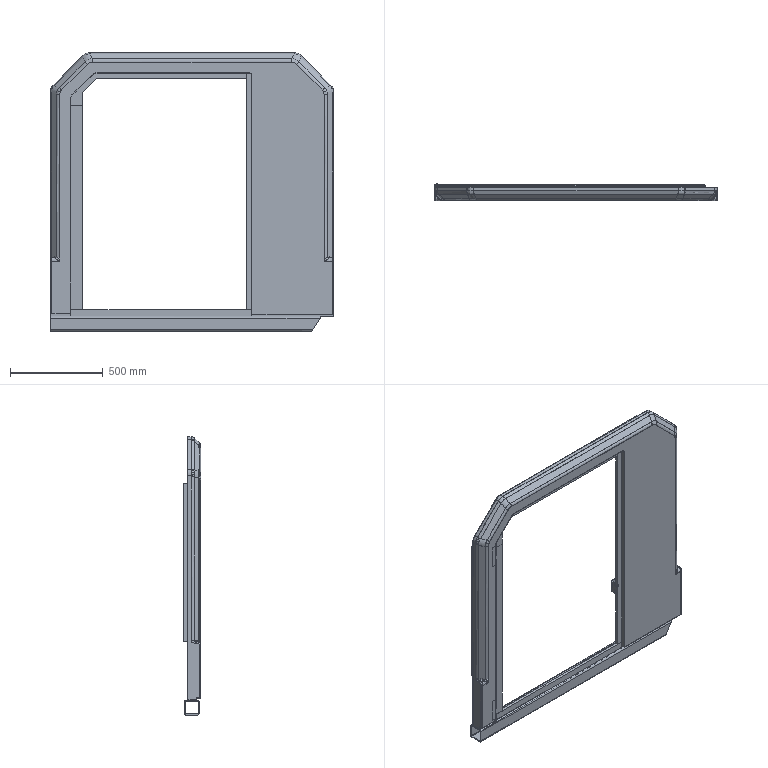Part | NX | features BREP 10 | 14 solids | 493 faces | box 1528 x 92.834 x 1503 mm | volume 9597800 mm3 | plane 245 | spline 134 | cylinder 90 | cone 24 | commonest cylinder face diameters 8 x16 9 x16 10 x15 20 x15 6 x8 13 x8